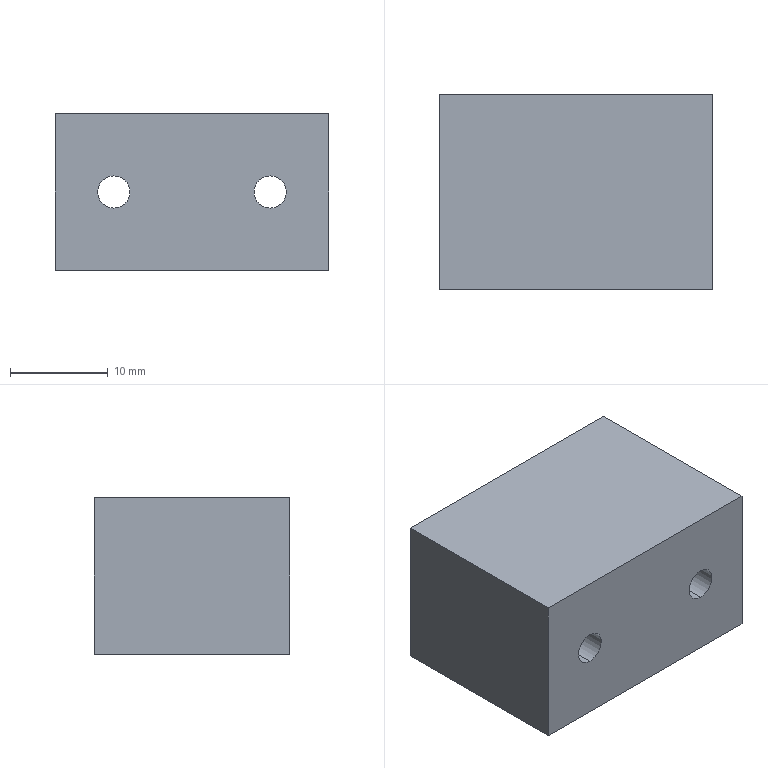Part | SolidWorks | features Extrusion 1, ICE 1 | 1 solid | 10 faces | box 28 x 20 x 16 mm | volume 8618 mm3 | plane 6 | cylinder 4 | commonest cylinder face diameters 3.3 x4
STEP:
#1=CARTESIAN_POINT('',(-8.,-10.,1.65));
#2=VERTEX_POINT('',#1);
#3=CARTESIAN_POINT('',(-8.,-10.,-1.65));
#4=VERTEX_POINT('',#3);
#5=CARTESIAN_POINT('',(-8.,-10.,0.));
#6=DIRECTION('',(0.,-1.,0.));
#7=DIRECTION('',(0.,0.,-1.));
#8=AXIS2_PLACEMENT_3D('',#5,#6,#7);
#9=CIRCLE('',#8,1.65);
#10=EDGE_CURVE('',#2,#4,#9,.T.);
#11=ORIENTED_EDGE('',*,*,#10,.T.);
#12=CARTESIAN_POINT('',(-8.,10.,-1.65));
#13=VERTEX_POINT('',#12);
#14=CARTESIAN_POINT('',(-8.,-13.,-1.65));
#15=DIRECTION('',(0.,1.,0.));
#16=VECTOR('',#15,1000.);
#17=LINE('',#14,#16);
#18=EDGE_CURVE('',#4,#13,#17,.T.);
#19=ORIENTED_EDGE('',*,*,#18,.T.);
#20=CARTESIAN_POINT('',(-8.,10.,1.65));
#21=VERTEX_POINT('',#20);
#22=CARTESIAN_POINT('',(-8.,10.,0.));
#23=DIRECTION('',(0.,1.,0.));
#24=DIRECTION('',(0.,0.,1.));
#25=AXIS2_PLACEMENT_3D('',#22,#23,#24);
#26=CIRCLE('',#25,1.65);
#27=EDGE_CURVE('',#13,#21,#26,.T.);
#28=ORIENTED_EDGE('',*,*,#27,.T.);
#29=CARTESIAN_POINT('',(-8.,-13.,1.65));
#30=DIRECTION('',(0.,1.,0.));
#31=VECTOR('',#30,1000.);
#32=LINE('',#29,#31);
#33=EDGE_CURVE('',#2,#21,#32,.T.);
#34=ORIENTED_EDGE('',*,*,#33,.F.);
#35=EDGE_LOOP('',(#11,#19,#28,#34));
#36=FACE_OUTER_BOUND('',#35,.T.);
#37=CARTESIAN_POINT('',(-8.,-13.,0.));
#38=DIRECTION('',(0.,1.,0.));
#39=DIRECTION('',(0.,0.,1.));
#40=AXIS2_PLACEMENT_3D('',#37,#38,#39);
#41=CYLINDRICAL_SURFACE('',#40,1.65);
#42=ADVANCED_FACE('',(#36),#41,.F.);
#43=CARTESIAN_POINT('',(8.,-10.,1.65));
#44=VERTEX_POINT('',#43);
#45=CARTESIAN_POINT('',(8.,-10.,-1.65));
#46=VERTEX_POINT('',#45);
#47=CARTESIAN_POINT('',(8.,-10.,0.));
#48=DIRECTION('',(0.,-1.,0.));
#49=DIRECTION('',(0.,0.,-1.));
#50=AXIS2_PLACEMENT_3D('',#47,#48,#49);
#51=CIRCLE('',#50,1.65);
#52=EDGE_CURVE('',#44,#46,#51,.T.);
#53=ORIENTED_EDGE('',*,*,#52,.T.);
#54=CARTESIAN_POINT('',(8.,10.,-1.65));
#55=VERTEX_POINT('',#54);
#56=CARTESIAN_POINT('',(8.,-13.,-1.65));
#57=DIRECTION('',(0.,1.,0.));
#58=VECTOR('',#57,1000.);
#59=LINE('',#56,#58);
#60=EDGE_CURVE('',#46,#55,#59,.T.);
#61=ORIENTED_EDGE('',*,*,#60,.T.);
#62=CARTESIAN_POINT('',(8.,10.,1.65));
#63=VERTEX_POINT('',#62);
#64=CARTESIAN_POINT('',(8.,10.,0.));
#65=DIRECTION('',(0.,1.,0.));
#66=DIRECTION('',(0.,0.,1.));
#67=AXIS2_PLACEMENT_3D('',#64,#65,#66);
#68=CIRCLE('',#67,1.65);
#69=EDGE_CURVE('',#55,#63,#68,.T.);
#70=ORIENTED_EDGE('',*,*,#69,.T.);
#71=CARTESIAN_POINT('',(8.,-13.,1.65));
#72=DIRECTION('',(0.,1.,0.));
#73=VECTOR('',#72,1000.);
#74=LINE('',#71,#73);
#75=EDGE_CURVE('',#44,#63,#74,.T.);
#76=ORIENTED_EDGE('',*,*,#75,.F.);
#77=EDGE_LOOP('',(#53,#61,#70,#76));
#78=FACE_OUTER_BOUND('',#77,.T.);
#79=CARTESIAN_POINT('',(8.,-13.,0.));
#80=DIRECTION('',(0.,1.,0.));
#81=DIRECTION('',(0.,0.,1.));
#82=AXIS2_PLACEMENT_3D('',#79,#80,#81);
#83=CYLINDRICAL_SURFACE('',#82,1.65);
#84=ADVANCED_FACE('',(#78),#83,.F.);
#85=CARTESIAN_POINT('',(-14.,10.,8.));
#86=VERTEX_POINT('',#85);
#87=CARTESIAN_POINT('',(-14.,-10.,8.));
#88=VERTEX_POINT('',#87);
#89=CARTESIAN_POINT('',(-14.,10.,8.));
#90=DIRECTION('',(0.,-1.,0.));
#91=VECTOR('',#90,1000.);
#92=LINE('',#89,#91);
#93=EDGE_CURVE('',#86,#88,#92,.T.);
#94=ORIENTED_EDGE('',*,*,#93,.F.);
#95=CARTESIAN_POINT('',(-14.,10.,-8.));
#96=VERTEX_POINT('',#95);
#97=CARTESIAN_POINT('',(-14.,10.,-8.));
#98=DIRECTION('',(0.,0.,1.));
#99=VECTOR('',#98,1000.);
#100=LINE('',#97,#99);
#101=EDGE_CURVE('',#96,#86,#100,.T.);
#102=ORIENTED_EDGE('',*,*,#101,.F.);
#103=CARTESIAN_POINT('',(-14.,-10.,-8.));
#104=VERTEX_POINT('',#103);
#105=CARTESIAN_POINT('',(-14.,10.,-8.));
#106=DIRECTION('',(0.,-1.,0.));
#107=VECTOR('',#106,1000.);
#108=LINE('',#105,#107);
#109=EDGE_CURVE('',#96,#104,#108,.T.);
#110=ORIENTED_EDGE('',*,*,#109,.T.);
#111=CARTESIAN_POINT('',(-14.,-10.,-8.));
#112=DIRECTION('',(0.,0.,1.));
#113=VECTOR('',#112,1000.);
#114=LINE('',#111,#113);
#115=EDGE_CURVE('',#104,#88,#114,.T.);
#116=ORIENTED_EDGE('',*,*,#115,.T.);
#117=EDGE_LOOP('',(#94,#102,#110,#116));
#118=FACE_OUTER_BOUND('',#117,.T.);
#119=CARTESIAN_POINT('',(-14.,10.,-8.));
#120=DIRECTION('',(-1.,0.,0.));
#121=DIRECTION('',(0.,0.,1.));
#122=AXIS2_PLACEMENT_3D('',#119,#120,#121);
#123=PLANE('',#122);
#124=ADVANCED_FACE('',(#118),#123,.T.);
#125=CARTESIAN_POINT('',(-8.,10.,0.));
#126=DIRECTION('',(0.,1.,0.));
#127=DIRECTION('',(0.,0.,1.));
#128=AXIS2_PLACEMENT_3D('',#125,#126,#127);
#129=CIRCLE('',#128,1.65);
#130=EDGE_CURVE('',#21,#13,#129,.T.);
#131=ORIENTED_EDGE('',*,*,#130,.F.);
#132=ORIENTED_EDGE('',*,*,#27,.F.);
#133=EDGE_LOOP('',(#131,#132));
#134=FACE_BOUND('',#133,.T.);
#135=CARTESIAN_POINT('',(8.,10.,0.));
#136=DIRECTION('',(0.,1.,0.));
#137=DIRECTION('',(0.,0.,1.));
#138=AXIS2_PLACEMENT_3D('',#135,#136,#137);
#139=CIRCLE('',#138,1.65);
#140=EDGE_CURVE('',#63,#55,#139,.T.);
#141=ORIENTED_EDGE('',*,*,#140,.F.);
#142=ORIENTED_EDGE('',*,*,#69,.F.);
#143=EDGE_LOOP('',(#141,#142));
#144=FACE_BOUND('',#143,.T.);
#145=CARTESIAN_POINT('',(14.,10.,8.));
#146=VERTEX_POINT('',#145);
#147=CARTESIAN_POINT('',(14.,10.,8.));
#148=DIRECTION('',(-1.,0.,0.));
#149=VECTOR('',#148,1000.);
#150=LINE('',#147,#149);
#151=EDGE_CURVE('',#146,#86,#150,.T.);
#152=ORIENTED_EDGE('',*,*,#151,.F.);
#153=CARTESIAN_POINT('',(14.,10.,-8.));
#154=VERTEX_POINT('',#153);
#155=CARTESIAN_POINT('',(14.,10.,-8.));
#156=DIRECTION('',(0.,0.,1.));
#157=VECTOR('',#156,1000.);
#158=LINE('',#155,#157);
#159=EDGE_CURVE('',#154,#146,#158,.T.);
#160=ORIENTED_EDGE('',*,*,#159,.F.);
#161=CARTESIAN_POINT('',(14.,10.,-8.));
#162=DIRECTION('',(-1.,0.,0.));
#163=VECTOR('',#162,1000.);
#164=LINE('',#161,#163);
#165=EDGE_CURVE('',#154,#96,#164,.T.);
#166=ORIENTED_EDGE('',*,*,#165,.T.);
#167=ORIENTED_EDGE('',*,*,#101,.T.);
#168=EDGE_LOOP('',(#152,#160,#166,#167));
#169=FACE_OUTER_BOUND('',#168,.T.);
#170=CARTESIAN_POINT('',(14.,10.,-8.));
#171=DIRECTION('',(0.,1.,0.));
#172=DIRECTION('',(0.,0.,1.));
#173=AXIS2_PLACEMENT_3D('',#170,#171,#172);
#174=PLANE('',#173);
#175=ADVANCED_FACE('',(#134,#144,#169),#174,.T.);
#176=CARTESIAN_POINT('',(14.,-10.,8.));
#177=VERTEX_POINT('',#176);
#178=CARTESIAN_POINT('',(14.,-10.,8.));
#179=DIRECTION('',(0.,1.,0.));
#180=VECTOR('',#179,1000.);
#181=LINE('',#178,#180);
#182=EDGE_CURVE('',#177,#146,#181,.T.);
#183=ORIENTED_EDGE('',*,*,#182,.F.);
#184=CARTESIAN_POINT('',(14.,-10.,-8.));
#185=VERTEX_POINT('',#184);
#186=CARTESIAN_POINT('',(14.,-10.,-8.));
#187=DIRECTION('',(0.,0.,1.));
#188=VECTOR('',#187,1000.);
#189=LINE('',#186,#188);
#190=EDGE_CURVE('',#185,#177,#189,.T.);
#191=ORIENTED_EDGE('',*,*,#190,.F.);
#192=CARTESIAN_POINT('',(14.,-10.,-8.));
#193=DIRECTION('',(0.,1.,0.));
#194=VECTOR('',#193,1000.);
#195=LINE('',#192,#194);
#196=EDGE_CURVE('',#185,#154,#195,.T.);
#197=ORIENTED_EDGE('',*,*,#196,.T.);
#198=ORIENTED_EDGE('',*,*,#159,.T.);
#199=EDGE_LOOP('',(#183,#191,#197,#198));
#200=FACE_OUTER_BOUND('',#199,.T.);
#201=CARTESIAN_POINT('',(14.,-10.,-8.));
#202=DIRECTION('',(1.,0.,0.));
#203=DIRECTION('',(0.,0.,-1.));
#204=AXIS2_PLACEMENT_3D('',#201,#202,#203);
#205=PLANE('',#204);
#206=ADVANCED_FACE('',(#200),#205,.T.);
#207=ORIENTED_EDGE('',*,*,#10,.F.);
#208=CARTESIAN_POINT('',(-8.,-10.,0.));
#209=DIRECTION('',(0.,-1.,0.));
#210=DIRECTION('',(0.,0.,-1.));
#211=AXIS2_PLACEMENT_3D('',#208,#209,#210);
#212=CIRCLE('',#211,1.65);
#213=EDGE_CURVE('',#4,#2,#212,.T.);
#214=ORIENTED_EDGE('',*,*,#213,.F.);
#215=EDGE_LOOP('',(#207,#214));
#216=FACE_BOUND('',#215,.T.);
#217=ORIENTED_EDGE('',*,*,#52,.F.);
#218=CARTESIAN_POINT('',(8.,-10.,0.));
#219=DIRECTION('',(0.,-1.,0.));
#220=DIRECTION('',(0.,0.,-1.));
#221=AXIS2_PLACEMENT_3D('',#218,#219,#220);
#222=CIRCLE('',#221,1.65);
#223=EDGE_CURVE('',#46,#44,#222,.T.);
#224=ORIENTED_EDGE('',*,*,#223,.F.);
#225=EDGE_LOOP('',(#217,#224));
#226=FACE_BOUND('',#225,.T.);
#227=CARTESIAN_POINT('',(-14.,-10.,8.));
#228=DIRECTION('',(1.,0.,0.));
#229=VECTOR('',#228,1000.);
#230=LINE('',#227,#229);
#231=EDGE_CURVE('',#88,#177,#230,.T.);
#232=ORIENTED_EDGE('',*,*,#231,.F.);
#233=ORIENTED_EDGE('',*,*,#115,.F.);
#234=CARTESIAN_POINT('',(-14.,-10.,-8.));
#235=DIRECTION('',(1.,0.,0.));
#236=VECTOR('',#235,1000.);
#237=LINE('',#234,#236);
#238=EDGE_CURVE('',#104,#185,#237,.T.);
#239=ORIENTED_EDGE('',*,*,#238,.T.);
#240=ORIENTED_EDGE('',*,*,#190,.T.);
#241=EDGE_LOOP('',(#232,#233,#239,#240));
#242=FACE_OUTER_BOUND('',#241,.T.);
#243=CARTESIAN_POINT('',(-14.,-10.,-8.));
#244=DIRECTION('',(0.,-1.,0.));
#245=DIRECTION('',(0.,0.,-1.));
#246=AXIS2_PLACEMENT_3D('',#243,#244,#245);
#247=PLANE('',#246);
#248=ADVANCED_FACE('',(#216,#226,#242),#247,.T.);
#249=ORIENTED_EDGE('',*,*,#109,.F.);
#250=ORIENTED_EDGE('',*,*,#165,.F.);
#251=ORIENTED_EDGE('',*,*,#196,.F.);
#252=ORIENTED_EDGE('',*,*,#238,.F.);
#253=EDGE_LOOP('',(#249,#250,#251,#252));
#254=FACE_OUTER_BOUND('',#253,.T.);
#255=CARTESIAN_POINT('',(0.,0.,-8.));
#256=DIRECTION('',(0.,0.,1.));
#257=DIRECTION('',(1.,0.,0.));
#258=AXIS2_PLACEMENT_3D('',#255,#256,#257);
#259=PLANE('',#258);
#260=ADVANCED_FACE('',(#254),#259,.F.);
#261=ORIENTED_EDGE('',*,*,#93,.T.);
#262=ORIENTED_EDGE('',*,*,#231,.T.);
#263=ORIENTED_EDGE('',*,*,#182,.T.);
#264=ORIENTED_EDGE('',*,*,#151,.T.);
#265=EDGE_LOOP('',(#261,#262,#263,#264));
#266=FACE_OUTER_BOUND('',#265,.T.);
#267=CARTESIAN_POINT('',(0.,0.,8.));
#268=DIRECTION('',(0.,0.,1.));
#269=DIRECTION('',(1.,0.,0.));
#270=AXIS2_PLACEMENT_3D('',#267,#268,#269);
#271=PLANE('',#270);
#272=ADVANCED_FACE('',(#266),#271,.T.);
#273=ORIENTED_EDGE('',*,*,#60,.F.);
#274=ORIENTED_EDGE('',*,*,#223,.T.);
#275=ORIENTED_EDGE('',*,*,#75,.T.);
#276=ORIENTED_EDGE('',*,*,#140,.T.);
#277=EDGE_LOOP('',(#273,#274,#275,#276));
#278=FACE_OUTER_BOUND('',#277,.T.);
#279=CARTESIAN_POINT('',(8.,-13.,0.));
#280=DIRECTION('',(0.,1.,0.));
#281=DIRECTION('',(0.,0.,1.));
#282=AXIS2_PLACEMENT_3D('',#279,#280,#281);
#283=CYLINDRICAL_SURFACE('',#282,1.65);
#284=ADVANCED_FACE('',(#278),#283,.F.);
#285=ORIENTED_EDGE('',*,*,#18,.F.);
#286=ORIENTED_EDGE('',*,*,#213,.T.);
#287=ORIENTED_EDGE('',*,*,#33,.T.);
#288=ORIENTED_EDGE('',*,*,#130,.T.);
#289=EDGE_LOOP('',(#285,#286,#287,#288));
#290=FACE_OUTER_BOUND('',#289,.T.);
#291=CARTESIAN_POINT('',(-8.,-13.,0.));
#292=DIRECTION('',(0.,1.,0.));
#293=DIRECTION('',(0.,0.,1.));
#294=AXIS2_PLACEMENT_3D('',#291,#292,#293);
#295=CYLINDRICAL_SURFACE('',#294,1.65);
#296=ADVANCED_FACE('',(#290),#295,.F.);
#297=CLOSED_SHELL('',(#42,#84,#124,#175,#206,#248,#260,#272,#284,#296));
#298=MANIFOLD_SOLID_BREP('',#297);
#299=CARTESIAN_POINT('',(0.,0.,0.));
#300=DIRECTION('',(0.,0.,1.));
#301=DIRECTION('',(1.,0.,0.));
#302=AXIS2_PLACEMENT_3D('',#299,#300,#301);
#303=(LENGTH_UNIT()NAMED_UNIT(*)SI_UNIT(.MILLI.,.METRE.));
#304=UNCERTAINTY_MEASURE_WITH_UNIT(LENGTH_MEASURE(0.00001),#303,'','');
#305=(NAMED_UNIT(*)PLANE_ANGLE_UNIT()SI_UNIT($,.RADIAN.));
#306=(NAMED_UNIT(*)SI_UNIT($,.STERADIAN.)SOLID_ANGLE_UNIT());
#307=(GEOMETRIC_REPRESENTATION_CONTEXT(3)GLOBAL_UNCERTAINTY_ASSIGNED_CONTEXT((#304))GLOBAL_UNIT_ASSIGNED_CONTEXT((#303,#305,#306))REPRESENTATION_CONTEXT('',''));
#308=ADVANCED_BREP_SHAPE_REPRESENTATION('',(#298,#302),#307);